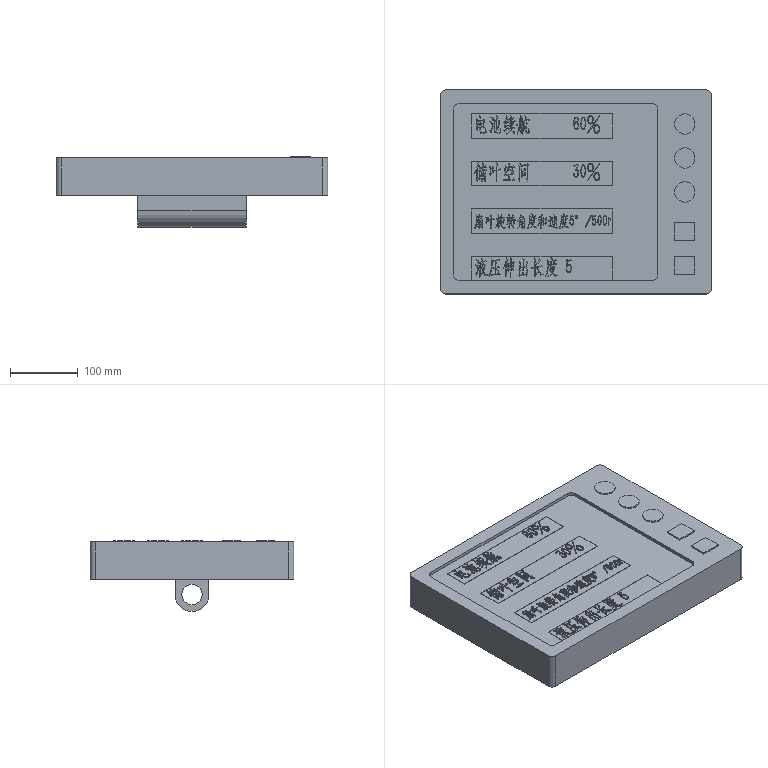Part | SolidWorks | features ICE 7, Extrusion 1, Fillet 1, HoleWzd 1 | 1 solid | 2609 faces | box 400 x 300 x 104.5 mm | volume 6453312 mm3 | plane 1783 | spline 801 | cylinder 21 | cone 4 | commonest cylinder face diameters 16 x8 30 x8 14 x4 50 x1